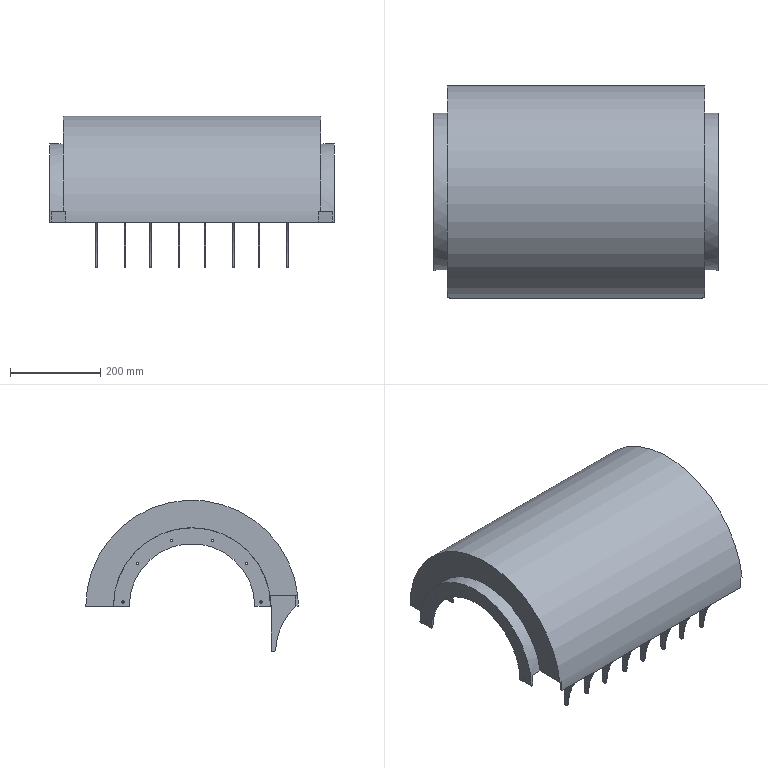Part | SolidWorks | features BaseBody 1 | 1 solid | 112 faces | box 630 x 470 x 335 mm | volume 3643820 mm3 | cylinder 72 | plane 40 | commonest cylinder face diameters 5 x24 10.092 x16 460 x9 267.222 x8 350 x8 277.768 x2